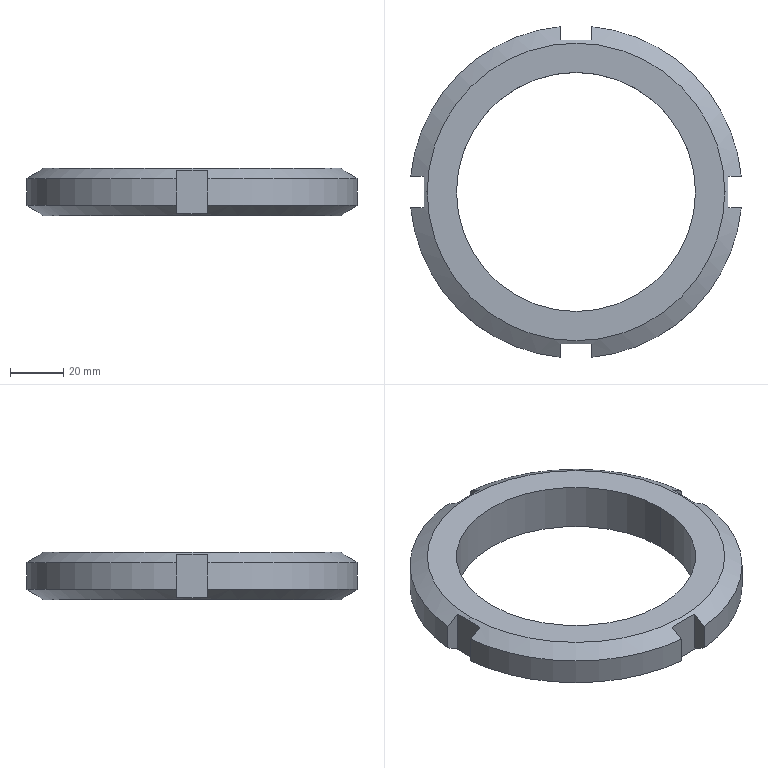Part | SolidWorks | features Extrusion 1, ICE 1, RevCut 1 | 1 solid | 24 faces | box 124.423 x 124.423 x 18 mm | volume 93238 mm3 | plane 14 | cylinder 6 | cone 4 | commonest cylinder face diameters 125 x4 90 x2
STEP:
#1=CARTESIAN_POINT('',(-56.,0.,18.));
#2=VERTEX_POINT('',#1);
#3=CARTESIAN_POINT('',(56.,0.,18.));
#4=VERTEX_POINT('',#3);
#5=CARTESIAN_POINT('',(0.,0.,18.));
#6=DIRECTION('',(0.,0.,-1.));
#7=DIRECTION('',(-1.,0.,0.));
#8=AXIS2_PLACEMENT_3D('',#5,#6,#7);
#9=CIRCLE('',#8,56.);
#10=EDGE_CURVE('',#2,#4,#9,.T.);
#11=ORIENTED_EDGE('',*,*,#10,.T.);
#12=CARTESIAN_POINT('',(57.211,0.,17.255));
#13=VERTEX_POINT('',#12);
#14=CARTESIAN_POINT('',(62.5,0.,14.));
#15=DIRECTION('',(0.8517,0.,-0.5241));
#16=VECTOR('',#15,1000.);
#17=LINE('',#14,#16);
#18=EDGE_CURVE('',#4,#13,#17,.T.);
#19=ORIENTED_EDGE('',*,*,#18,.T.);
#20=CARTESIAN_POINT('',(57.211,6.,17.061));
#21=VERTEX_POINT('',#20);
#22=CARTESIAN_POINT('',(57.211,6.,17.061));
#23=CARTESIAN_POINT('',(57.211,4.005,17.19));
#24=CARTESIAN_POINT('',(57.211,2.005,17.255));
#25=CARTESIAN_POINT('',(57.211,0.,17.255));
#26=B_SPLINE_CURVE_WITH_KNOTS('',3,(#22,#23,#24,#25),.UNSPECIFIED.,.F.,.F.,(4,4),(0.0144,0.02039),.UNSPECIFIED.);
#27=EDGE_CURVE('',#21,#13,#26,.T.);
#28=ORIENTED_EDGE('',*,*,#27,.F.);
#29=CARTESIAN_POINT('',(62.211,6.,14.));
#30=VERTEX_POINT('',#29);
#31=CARTESIAN_POINT('',(62.211,6.,14.));
#32=CARTESIAN_POINT('',(61.305,6.,14.555));
#33=CARTESIAN_POINT('',(60.399,6.,15.11));
#34=CARTESIAN_POINT('',(59.493,6.,15.665));
#35=CARTESIAN_POINT('',(58.733,6.,16.13));
#36=CARTESIAN_POINT('',(57.972,6.,16.596));
#37=CARTESIAN_POINT('',(57.211,6.,17.061));
#38=B_SPLINE_CURVE_WITH_KNOTS('',3,(#31,#32,#33,#34,#35,#36,#37),.UNSPECIFIED.,.F.,.F.,(4,3,4),(0.008854,0.01204,0.01472),.UNSPECIFIED.);
#39=EDGE_CURVE('',#30,#21,#38,.T.);
#40=ORIENTED_EDGE('',*,*,#39,.F.);
#41=CARTESIAN_POINT('',(6.,62.211,14.));
#42=VERTEX_POINT('',#41);
#43=CARTESIAN_POINT('',(0.,0.,14.));
#44=DIRECTION('',(0.,0.,-1.));
#45=DIRECTION('',(-1.,0.,0.));
#46=AXIS2_PLACEMENT_3D('',#43,#44,#45);
#47=CIRCLE('',#46,62.5);
#48=EDGE_CURVE('',#42,#30,#47,.T.);
#49=ORIENTED_EDGE('',*,*,#48,.F.);
#50=CARTESIAN_POINT('',(6.,57.211,17.061));
#51=VERTEX_POINT('',#50);
#52=CARTESIAN_POINT('',(6.,57.211,17.061));
#53=CARTESIAN_POINT('',(6.,57.972,16.596));
#54=CARTESIAN_POINT('',(6.,58.733,16.13));
#55=CARTESIAN_POINT('',(6.,59.493,15.665));
#56=CARTESIAN_POINT('',(6.,60.399,15.11));
#57=CARTESIAN_POINT('',(6.,61.305,14.555));
#58=CARTESIAN_POINT('',(6.,62.211,14.));
#59=B_SPLINE_CURVE_WITH_KNOTS('',3,(#52,#53,#54,#55,#56,#57,#58),.UNSPECIFIED.,.F.,.F.,(4,3,4),(0.009366,0.01204,0.01523),.UNSPECIFIED.);
#60=EDGE_CURVE('',#51,#42,#59,.T.);
#61=ORIENTED_EDGE('',*,*,#60,.F.);
#62=CARTESIAN_POINT('',(-6.,57.211,17.061));
#63=VERTEX_POINT('',#62);
#64=CARTESIAN_POINT('',(-6.,57.211,17.061));
#65=CARTESIAN_POINT('',(-4.998,57.211,17.126));
#66=CARTESIAN_POINT('',(-3.993,57.211,17.174));
#67=CARTESIAN_POINT('',(-1.987,57.211,17.239));
#68=CARTESIAN_POINT('',(-0.9858,57.211,17.255));
#69=CARTESIAN_POINT('',(2.015,57.211,17.254));
#70=CARTESIAN_POINT('',(4.01,57.211,17.189));
#71=CARTESIAN_POINT('',(6.,57.211,17.061));
#72=B_SPLINE_CURVE_WITH_KNOTS('',3,(#64,#65,#66,#67,#68,#69,#70,#71),.UNSPECIFIED.,.F.,.F.,(4,2,2,4),(0.02345,0.02644,0.02944,0.03543),.UNSPECIFIED.);
#73=EDGE_CURVE('',#63,#51,#72,.T.);
#74=ORIENTED_EDGE('',*,*,#73,.F.);
#75=CARTESIAN_POINT('',(-6.,62.211,14.));
#76=VERTEX_POINT('',#75);
#77=CARTESIAN_POINT('',(-6.,62.211,14.));
#78=CARTESIAN_POINT('',(-6.,61.305,14.555));
#79=CARTESIAN_POINT('',(-6.,60.399,15.11));
#80=CARTESIAN_POINT('',(-6.,59.493,15.665));
#81=CARTESIAN_POINT('',(-6.,58.733,16.13));
#82=CARTESIAN_POINT('',(-6.,57.972,16.596));
#83=CARTESIAN_POINT('',(-6.,57.211,17.061));
#84=B_SPLINE_CURVE_WITH_KNOTS('',3,(#77,#78,#79,#80,#81,#82,#83),.UNSPECIFIED.,.F.,.F.,(4,3,4),(0.008854,0.01204,0.01472),.UNSPECIFIED.);
#85=EDGE_CURVE('',#76,#63,#84,.T.);
#86=ORIENTED_EDGE('',*,*,#85,.F.);
#87=CARTESIAN_POINT('',(-62.211,6.,14.));
#88=VERTEX_POINT('',#87);
#89=CARTESIAN_POINT('',(0.,0.,14.));
#90=DIRECTION('',(0.,0.,-1.));
#91=DIRECTION('',(-1.,0.,0.));
#92=AXIS2_PLACEMENT_3D('',#89,#90,#91);
#93=CIRCLE('',#92,62.5);
#94=EDGE_CURVE('',#88,#76,#93,.T.);
#95=ORIENTED_EDGE('',*,*,#94,.F.);
#96=CARTESIAN_POINT('',(-57.211,6.,17.061));
#97=VERTEX_POINT('',#96);
#98=CARTESIAN_POINT('',(-57.211,6.,17.061));
#99=CARTESIAN_POINT('',(-58.578,6.,16.225));
#100=CARTESIAN_POINT('',(-59.945,6.,15.388));
#101=CARTESIAN_POINT('',(-61.311,6.,14.551));
#102=CARTESIAN_POINT('',(-61.611,6.,14.367));
#103=CARTESIAN_POINT('',(-61.911,6.,14.184));
#104=CARTESIAN_POINT('',(-62.211,6.,14.));
#105=B_SPLINE_CURVE_WITH_KNOTS('',3,(#98,#99,#100,#101,#102,#103,#104),.UNSPECIFIED.,.F.,.F.,(4,3,4),(0.007234,0.01204,0.0131),.UNSPECIFIED.);
#106=EDGE_CURVE('',#97,#88,#105,.T.);
#107=ORIENTED_EDGE('',*,*,#106,.F.);
#108=CARTESIAN_POINT('',(-57.211,0.,17.255));
#109=VERTEX_POINT('',#108);
#110=CARTESIAN_POINT('',(-57.211,0.,17.255));
#111=CARTESIAN_POINT('',(-57.211,2.005,17.255));
#112=CARTESIAN_POINT('',(-57.211,4.005,17.19));
#113=CARTESIAN_POINT('',(-57.211,6.,17.061));
#114=B_SPLINE_CURVE_WITH_KNOTS('',3,(#110,#111,#112,#113),.UNSPECIFIED.,.F.,.F.,(4,4),(0.02943,0.03543),.UNSPECIFIED.);
#115=EDGE_CURVE('',#109,#97,#114,.T.);
#116=ORIENTED_EDGE('',*,*,#115,.F.);
#117=CARTESIAN_POINT('',(-62.5,0.,14.));
#118=DIRECTION('',(-0.8517,0.,-0.5241));
#119=VECTOR('',#118,1000.);
#120=LINE('',#117,#119);
#121=EDGE_CURVE('',#2,#109,#120,.T.);
#122=ORIENTED_EDGE('',*,*,#121,.F.);
#123=EDGE_LOOP('',(#11,#19,#28,#40,#49,#61,#74,#86,#95,#107,#116,#122));
#124=FACE_OUTER_BOUND('',#123,.T.);
#125=CARTESIAN_POINT('',(0.,0.,14.));
#126=DIRECTION('',(0.,0.,-1.));
#127=DIRECTION('',(-1.,0.,0.));
#128=AXIS2_PLACEMENT_3D('',#125,#126,#127);
#129=CONICAL_SURFACE('',#128,62.5,1.019);
#130=ADVANCED_FACE('',(#124),#129,.T.);
#131=CARTESIAN_POINT('',(-56.,0.,0.));
#132=VERTEX_POINT('',#131);
#133=CARTESIAN_POINT('',(56.,0.,0.));
#134=VERTEX_POINT('',#133);
#135=CARTESIAN_POINT('',(0.,0.,0.));
#136=DIRECTION('',(0.,0.,-1.));
#137=DIRECTION('',(-1.,0.,0.));
#138=AXIS2_PLACEMENT_3D('',#135,#136,#137);
#139=CIRCLE('',#138,56.);
#140=EDGE_CURVE('',#132,#134,#139,.T.);
#141=ORIENTED_EDGE('',*,*,#140,.F.);
#142=CARTESIAN_POINT('',(-57.211,0.,0.7454));
#143=VERTEX_POINT('',#142);
#144=CARTESIAN_POINT('',(-56.,0.,0.));
#145=DIRECTION('',(-0.8517,0.,0.5241));
#146=VECTOR('',#145,1000.);
#147=LINE('',#144,#146);
#148=EDGE_CURVE('',#132,#143,#147,.T.);
#149=ORIENTED_EDGE('',*,*,#148,.T.);
#150=CARTESIAN_POINT('',(-57.211,6.,0.9385));
#151=VERTEX_POINT('',#150);
#152=CARTESIAN_POINT('',(-57.211,6.,0.9385));
#153=CARTESIAN_POINT('',(-57.211,4.005,0.8105));
#154=CARTESIAN_POINT('',(-57.211,2.005,0.7454));
#155=CARTESIAN_POINT('',(-57.211,0.,0.7454));
#156=B_SPLINE_CURVE_WITH_KNOTS('',3,(#152,#153,#154,#155),.UNSPECIFIED.,.F.,.F.,(4,4),(0.0144,0.02039),.UNSPECIFIED.);
#157=EDGE_CURVE('',#151,#143,#156,.T.);
#158=ORIENTED_EDGE('',*,*,#157,.F.);
#159=CARTESIAN_POINT('',(-62.211,6.,4.));
#160=VERTEX_POINT('',#159);
#161=CARTESIAN_POINT('',(-62.211,6.,4.));
#162=CARTESIAN_POINT('',(-61.911,6.,3.816));
#163=CARTESIAN_POINT('',(-61.611,6.,3.633));
#164=CARTESIAN_POINT('',(-61.311,6.,3.449));
#165=CARTESIAN_POINT('',(-59.945,6.,2.612));
#166=CARTESIAN_POINT('',(-58.578,6.,1.775));
#167=CARTESIAN_POINT('',(-57.211,6.,0.9385));
#168=B_SPLINE_CURVE_WITH_KNOTS('',3,(#161,#162,#163,#164,#165,#166,#167),.UNSPECIFIED.,.F.,.F.,(4,3,4),(0.01099,0.01204,0.01685),.UNSPECIFIED.);
#169=EDGE_CURVE('',#160,#151,#168,.T.);
#170=ORIENTED_EDGE('',*,*,#169,.F.);
#171=CARTESIAN_POINT('',(-6.,62.211,4.));
#172=VERTEX_POINT('',#171);
#173=CARTESIAN_POINT('',(0.,0.,4.));
#174=DIRECTION('',(0.,0.,-1.));
#175=DIRECTION('',(-1.,0.,0.));
#176=AXIS2_PLACEMENT_3D('',#173,#174,#175);
#177=CIRCLE('',#176,62.5);
#178=EDGE_CURVE('',#160,#172,#177,.T.);
#179=ORIENTED_EDGE('',*,*,#178,.T.);
#180=CARTESIAN_POINT('',(-6.,57.211,0.9385));
#181=VERTEX_POINT('',#180);
#182=CARTESIAN_POINT('',(-6.,57.211,0.9385));
#183=CARTESIAN_POINT('',(-6.,57.372,1.037));
#184=CARTESIAN_POINT('',(-6.,57.533,1.135));
#185=CARTESIAN_POINT('',(-6.,57.693,1.234));
#186=CARTESIAN_POINT('',(-6.,59.2,2.155));
#187=CARTESIAN_POINT('',(-6.,60.705,3.078));
#188=CARTESIAN_POINT('',(-6.,62.211,4.));
#189=B_SPLINE_CURVE_WITH_KNOTS('',3,(#182,#183,#184,#185,#186,#187,#188),.UNSPECIFIED.,.F.,.F.,(4,3,4),(0.01148,0.01204,0.01734),.UNSPECIFIED.);
#190=EDGE_CURVE('',#181,#172,#189,.T.);
#191=ORIENTED_EDGE('',*,*,#190,.F.);
#192=CARTESIAN_POINT('',(6.,57.211,0.9385));
#193=VERTEX_POINT('',#192);
#194=CARTESIAN_POINT('',(6.,57.211,0.9385));
#195=CARTESIAN_POINT('',(4.01,57.211,0.8108));
#196=CARTESIAN_POINT('',(2.015,57.211,0.7457));
#197=CARTESIAN_POINT('',(-0.9858,57.211,0.7453));
#198=CARTESIAN_POINT('',(-1.987,57.211,0.7613));
#199=CARTESIAN_POINT('',(-3.993,57.211,0.8257));
#200=CARTESIAN_POINT('',(-4.998,57.211,0.8742));
#201=CARTESIAN_POINT('',(-6.,57.211,0.9385));
#202=B_SPLINE_CURVE_WITH_KNOTS('',3,(#194,#195,#196,#197,#198,#199,#200,#201),.UNSPECIFIED.,.F.,.F.,(4,2,2,4),(0.0144,0.02038,0.02337,0.02636),.UNSPECIFIED.);
#203=EDGE_CURVE('',#193,#181,#202,.T.);
#204=ORIENTED_EDGE('',*,*,#203,.F.);
#205=CARTESIAN_POINT('',(6.,62.211,4.));
#206=VERTEX_POINT('',#205);
#207=CARTESIAN_POINT('',(6.,62.211,4.));
#208=CARTESIAN_POINT('',(6.,60.705,3.078));
#209=CARTESIAN_POINT('',(6.,59.2,2.155));
#210=CARTESIAN_POINT('',(6.,57.693,1.234));
#211=CARTESIAN_POINT('',(6.,57.533,1.135));
#212=CARTESIAN_POINT('',(6.,57.372,1.037));
#213=CARTESIAN_POINT('',(6.,57.211,0.9385));
#214=B_SPLINE_CURVE_WITH_KNOTS('',3,(#207,#208,#209,#210,#211,#212,#213),.UNSPECIFIED.,.F.,.F.,(4,3,4),(0.006744,0.01204,0.01261),.UNSPECIFIED.);
#215=EDGE_CURVE('',#206,#193,#214,.T.);
#216=ORIENTED_EDGE('',*,*,#215,.F.);
#217=CARTESIAN_POINT('',(62.211,6.,4.));
#218=VERTEX_POINT('',#217);
#219=CARTESIAN_POINT('',(0.,0.,4.));
#220=DIRECTION('',(0.,0.,-1.));
#221=DIRECTION('',(-1.,0.,0.));
#222=AXIS2_PLACEMENT_3D('',#219,#220,#221);
#223=CIRCLE('',#222,62.5);
#224=EDGE_CURVE('',#206,#218,#223,.T.);
#225=ORIENTED_EDGE('',*,*,#224,.T.);
#226=CARTESIAN_POINT('',(57.211,6.,0.9385));
#227=VERTEX_POINT('',#226);
#228=CARTESIAN_POINT('',(57.211,6.,0.9385));
#229=CARTESIAN_POINT('',(57.372,6.,1.037));
#230=CARTESIAN_POINT('',(57.533,6.,1.135));
#231=CARTESIAN_POINT('',(57.693,6.,1.234));
#232=CARTESIAN_POINT('',(59.2,6.,2.155));
#233=CARTESIAN_POINT('',(60.705,6.,3.078));
#234=CARTESIAN_POINT('',(62.211,6.,4.));
#235=B_SPLINE_CURVE_WITH_KNOTS('',3,(#228,#229,#230,#231,#232,#233,#234),.UNSPECIFIED.,.F.,.F.,(4,3,4),(0.01148,0.01204,0.01734),.UNSPECIFIED.);
#236=EDGE_CURVE('',#227,#218,#235,.T.);
#237=ORIENTED_EDGE('',*,*,#236,.F.);
#238=CARTESIAN_POINT('',(57.211,0.,0.7454));
#239=VERTEX_POINT('',#238);
#240=CARTESIAN_POINT('',(57.211,0.,0.7454));
#241=CARTESIAN_POINT('',(57.211,2.005,0.7454));
#242=CARTESIAN_POINT('',(57.211,4.005,0.8105));
#243=CARTESIAN_POINT('',(57.211,6.,0.9385));
#244=B_SPLINE_CURVE_WITH_KNOTS('',3,(#240,#241,#242,#243),.UNSPECIFIED.,.F.,.F.,(4,4),(0.02943,0.03543),.UNSPECIFIED.);
#245=EDGE_CURVE('',#239,#227,#244,.T.);
#246=ORIENTED_EDGE('',*,*,#245,.F.);
#247=CARTESIAN_POINT('',(56.,0.,0.));
#248=DIRECTION('',(0.8517,0.,0.5241));
#249=VECTOR('',#248,1000.);
#250=LINE('',#247,#249);
#251=EDGE_CURVE('',#134,#239,#250,.T.);
#252=ORIENTED_EDGE('',*,*,#251,.F.);
#253=EDGE_LOOP('',(#141,#149,#158,#170,#179,#191,#204,#216,#225,#237,#246,#252));
#254=FACE_OUTER_BOUND('',#253,.T.);
#255=CARTESIAN_POINT('',(0.,0.,0.));
#256=DIRECTION('',(0.,0.,1.));
#257=DIRECTION('',(1.,0.,0.));
#258=AXIS2_PLACEMENT_3D('',#255,#256,#257);
#259=CONICAL_SURFACE('',#258,56.,1.019);
#260=ADVANCED_FACE('',(#254),#259,.T.);
#261=CARTESIAN_POINT('',(-45.,0.,18.));
#262=VERTEX_POINT('',#261);
#263=CARTESIAN_POINT('',(45.,0.,18.));
#264=VERTEX_POINT('',#263);
#265=CARTESIAN_POINT('',(0.,0.,18.));
#266=DIRECTION('',(0.,0.,1.));
#267=DIRECTION('',(1.,0.,0.));
#268=AXIS2_PLACEMENT_3D('',#265,#266,#267);
#269=CIRCLE('',#268,45.);
#270=EDGE_CURVE('',#262,#264,#269,.T.);
#271=ORIENTED_EDGE('',*,*,#270,.T.);
#272=CARTESIAN_POINT('',(45.,0.,0.));
#273=VERTEX_POINT('',#272);
#274=CARTESIAN_POINT('',(45.,0.,18.));
#275=DIRECTION('',(0.,0.,-1.));
#276=VECTOR('',#275,1000.);
#277=LINE('',#274,#276);
#278=EDGE_CURVE('',#264,#273,#277,.T.);
#279=ORIENTED_EDGE('',*,*,#278,.T.);
#280=CARTESIAN_POINT('',(-45.,0.,0.));
#281=VERTEX_POINT('',#280);
#282=CARTESIAN_POINT('',(0.,0.,0.));
#283=DIRECTION('',(0.,0.,1.));
#284=DIRECTION('',(1.,0.,0.));
#285=AXIS2_PLACEMENT_3D('',#282,#283,#284);
#286=CIRCLE('',#285,45.);
#287=EDGE_CURVE('',#281,#273,#286,.T.);
#288=ORIENTED_EDGE('',*,*,#287,.F.);
#289=CARTESIAN_POINT('',(-45.,0.,18.));
#290=DIRECTION('',(0.,0.,-1.));
#291=VECTOR('',#290,1000.);
#292=LINE('',#289,#291);
#293=EDGE_CURVE('',#262,#281,#292,.T.);
#294=ORIENTED_EDGE('',*,*,#293,.F.);
#295=EDGE_LOOP('',(#271,#279,#288,#294));
#296=FACE_OUTER_BOUND('',#295,.T.);
#297=CARTESIAN_POINT('',(0.,0.,18.));
#298=DIRECTION('',(0.,0.,-1.));
#299=DIRECTION('',(-1.,0.,0.));
#300=AXIS2_PLACEMENT_3D('',#297,#298,#299);
#301=CYLINDRICAL_SURFACE('',#300,45.);
#302=ADVANCED_FACE('',(#296),#301,.F.);
#303=CARTESIAN_POINT('',(-6.,-62.211,14.));
#304=VERTEX_POINT('',#303);
#305=CARTESIAN_POINT('',(-62.211,-6.,14.));
#306=VERTEX_POINT('',#305);
#307=CARTESIAN_POINT('',(0.,0.,14.));
#308=DIRECTION('',(0.,0.,-1.));
#309=DIRECTION('',(-1.,0.,0.));
#310=AXIS2_PLACEMENT_3D('',#307,#308,#309);
#311=CIRCLE('',#310,62.5);
#312=EDGE_CURVE('',#304,#306,#311,.T.);
#313=ORIENTED_EDGE('',*,*,#312,.T.);
#314=CARTESIAN_POINT('',(-62.211,-6.,4.));
#315=VERTEX_POINT('',#314);
#316=CARTESIAN_POINT('',(-62.211,-6.,18.));
#317=DIRECTION('',(0.,0.,-1.));
#318=VECTOR('',#317,1000.);
#319=LINE('',#316,#318);
#320=EDGE_CURVE('',#306,#315,#319,.T.);
#321=ORIENTED_EDGE('',*,*,#320,.T.);
#322=CARTESIAN_POINT('',(-6.,-62.211,4.));
#323=VERTEX_POINT('',#322);
#324=CARTESIAN_POINT('',(0.,0.,4.));
#325=DIRECTION('',(0.,0.,-1.));
#326=DIRECTION('',(-1.,0.,0.));
#327=AXIS2_PLACEMENT_3D('',#324,#325,#326);
#328=CIRCLE('',#327,62.5);
#329=EDGE_CURVE('',#323,#315,#328,.T.);
#330=ORIENTED_EDGE('',*,*,#329,.F.);
#331=CARTESIAN_POINT('',(-6.,-62.211,18.));
#332=DIRECTION('',(0.,0.,-1.));
#333=VECTOR('',#332,1000.);
#334=LINE('',#331,#333);
#335=EDGE_CURVE('',#304,#323,#334,.T.);
#336=ORIENTED_EDGE('',*,*,#335,.F.);
#337=EDGE_LOOP('',(#313,#321,#330,#336));
#338=FACE_OUTER_BOUND('',#337,.T.);
#339=CARTESIAN_POINT('',(0.,0.,18.));
#340=DIRECTION('',(0.,0.,-1.));
#341=DIRECTION('',(-1.,0.,0.));
#342=AXIS2_PLACEMENT_3D('',#339,#340,#341);
#343=CYLINDRICAL_SURFACE('',#342,62.5);
#344=ADVANCED_FACE('',(#338),#343,.T.);
#345=CARTESIAN_POINT('',(62.211,-6.,14.));
#346=VERTEX_POINT('',#345);
#347=CARTESIAN_POINT('',(6.,-62.211,14.));
#348=VERTEX_POINT('',#347);
#349=CARTESIAN_POINT('',(0.,0.,14.));
#350=DIRECTION('',(0.,0.,-1.));
#351=DIRECTION('',(-1.,0.,0.));
#352=AXIS2_PLACEMENT_3D('',#349,#350,#351);
#353=CIRCLE('',#352,62.5);
#354=EDGE_CURVE('',#346,#348,#353,.T.);
#355=ORIENTED_EDGE('',*,*,#354,.T.);
#356=CARTESIAN_POINT('',(6.,-62.211,4.));
#357=VERTEX_POINT('',#356);
#358=CARTESIAN_POINT('',(6.,-62.211,18.));
#359=DIRECTION('',(0.,0.,-1.));
#360=VECTOR('',#359,1000.);
#361=LINE('',#358,#360);
#362=EDGE_CURVE('',#348,#357,#361,.T.);
#363=ORIENTED_EDGE('',*,*,#362,.T.);
#364=CARTESIAN_POINT('',(62.211,-6.,4.));
#365=VERTEX_POINT('',#364);
#366=CARTESIAN_POINT('',(0.,0.,4.));
#367=DIRECTION('',(0.,0.,-1.));
#368=DIRECTION('',(-1.,0.,0.));
#369=AXIS2_PLACEMENT_3D('',#366,#367,#368);
#370=CIRCLE('',#369,62.5);
#371=EDGE_CURVE('',#365,#357,#370,.T.);
#372=ORIENTED_EDGE('',*,*,#371,.F.);
#373=CARTESIAN_POINT('',(62.211,-6.,18.));
#374=DIRECTION('',(0.,0.,-1.));
#375=VECTOR('',#374,1000.);
#376=LINE('',#373,#375);
#377=EDGE_CURVE('',#346,#365,#376,.T.);
#378=ORIENTED_EDGE('',*,*,#377,.F.);
#379=EDGE_LOOP('',(#355,#363,#372,#378));
#380=FACE_OUTER_BOUND('',#379,.T.);
#381=CARTESIAN_POINT('',(0.,0.,18.));
#382=DIRECTION('',(0.,0.,-1.));
#383=DIRECTION('',(-1.,0.,0.));
#384=AXIS2_PLACEMENT_3D('',#381,#382,#383);
#385=CYLINDRICAL_SURFACE('',#384,62.5);
#386=ADVANCED_FACE('',(#380),#385,.T.);
#387=ORIENTED_EDGE('',*,*,#48,.T.);
#388=CARTESIAN_POINT('',(62.211,6.,18.));
#389=DIRECTION('',(0.,0.,-1.));
#390=VECTOR('',#389,1000.);
#391=LINE('',#388,#390);
#392=EDGE_CURVE('',#30,#218,#391,.T.);
#393=ORIENTED_EDGE('',*,*,#392,.T.);
#394=ORIENTED_EDGE('',*,*,#224,.F.);
#395=CARTESIAN_POINT('',(6.,62.211,18.));
#396=DIRECTION('',(0.,0.,-1.));
#397=VECTOR('',#396,1000.);
#398=LINE('',#395,#397);
#399=EDGE_CURVE('',#42,#206,#398,.T.);
#400=ORIENTED_EDGE('',*,*,#399,.F.);
#401=EDGE_LOOP('',(#387,#393,#394,#400));
#402=FACE_OUTER_BOUND('',#401,.T.);
#403=CARTESIAN_POINT('',(0.,0.,18.));
#404=DIRECTION('',(0.,0.,-1.));
#405=DIRECTION('',(-1.,0.,0.));
#406=AXIS2_PLACEMENT_3D('',#403,#404,#405);
#407=CYLINDRICAL_SURFACE('',#406,62.5);
#408=ADVANCED_FACE('',(#402),#407,.T.);
#409=ORIENTED_EDGE('',*,*,#178,.F.);
#410=CARTESIAN_POINT('',(-62.211,6.,18.));
#411=DIRECTION('',(0.,0.,-1.));
#412=VECTOR('',#411,1000.);
#413=LINE('',#410,#412);
#414=EDGE_CURVE('',#88,#160,#413,.T.);
#415=ORIENTED_EDGE('',*,*,#414,.F.);
#416=ORIENTED_EDGE('',*,*,#94,.T.);
#417=CARTESIAN_POINT('',(-6.,62.211,18.));
#418=DIRECTION('',(0.,0.,-1.));
#419=VECTOR('',#418,1000.);
#420=LINE('',#417,#419);
#421=EDGE_CURVE('',#76,#172,#420,.T.);
#422=ORIENTED_EDGE('',*,*,#421,.T.);
#423=EDGE_LOOP('',(#409,#415,#416,#422));
#424=FACE_OUTER_BOUND('',#423,.T.);
#425=CARTESIAN_POINT('',(0.,0.,18.));
#426=DIRECTION('',(0.,0.,-1.));
#427=DIRECTION('',(-1.,0.,0.));
#428=AXIS2_PLACEMENT_3D('',#425,#426,#427);
#429=CYLINDRICAL_SURFACE('',#428,62.5);
#430=ADVANCED_FACE('',(#424),#429,.T.);
#431=ORIENTED_EDGE('',*,*,#270,.F.);
#432=CARTESIAN_POINT('',(0.,0.,18.));
#433=DIRECTION('',(0.,0.,1.));
#434=DIRECTION('',(1.,0.,0.));
#435=AXIS2_PLACEMENT_3D('',#432,#433,#434);
#436=CIRCLE('',#435,45.);
#437=EDGE_CURVE('',#264,#262,#436,.T.);
#438=ORIENTED_EDGE('',*,*,#437,.F.);
#439=EDGE_LOOP('',(#431,#438));
#440=FACE_BOUND('',#439,.T.);
#441=ORIENTED_EDGE('',*,*,#10,.F.);
#442=CARTESIAN_POINT('',(0.,0.,18.));
#443=DIRECTION('',(0.,0.,-1.));
#444=DIRECTION('',(-1.,0.,0.));
#445=AXIS2_PLACEMENT_3D('',#442,#443,#444);
#446=CIRCLE('',#445,56.);
#447=EDGE_CURVE('',#4,#2,#446,.T.);
#448=ORIENTED_EDGE('',*,*,#447,.F.);
#449=EDGE_LOOP('',(#441,#448));
#450=FACE_OUTER_BOUND('',#449,.T.);
#451=CARTESIAN_POINT('',(0.,0.,18.));
#452=DIRECTION('',(0.,0.,1.));
#453=DIRECTION('',(1.,0.,0.));
#454=AXIS2_PLACEMENT_3D('',#451,#452,#453);
#455=PLANE('',#454);
#456=ADVANCED_FACE('',(#440,#450),#455,.T.);
#457=ORIENTED_EDGE('',*,*,#287,.T.);
#458=CARTESIAN_POINT('',(0.,0.,0.));
#459=DIRECTION('',(0.,0.,1.));
#460=DIRECTION('',(1.,0.,0.));
#461=AXIS2_PLACEMENT_3D('',#458,#459,#460);
#462=CIRCLE('',#461,45.);
#463=EDGE_CURVE('',#273,#281,#462,.T.);
#464=ORIENTED_EDGE('',*,*,#463,.T.);
#465=EDGE_LOOP('',(#457,#464));
#466=FACE_BOUND('',#465,.T.);
#467=CARTESIAN_POINT('',(0.,0.,0.));
#468=DIRECTION('',(0.,0.,-1.));
#469=DIRECTION('',(-1.,0.,0.));
#470=AXIS2_PLACEMENT_3D('',#467,#468,#469);
#471=CIRCLE('',#470,56.);
#472=EDGE_CURVE('',#134,#132,#471,.T.);
#473=ORIENTED_EDGE('',*,*,#472,.T.);
#474=ORIENTED_EDGE('',*,*,#140,.T.);
#475=EDGE_LOOP('',(#473,#474));
#476=FACE_OUTER_BOUND('',#475,.T.);
#477=CARTESIAN_POINT('',(0.,0.,0.));
#478=DIRECTION('',(0.,0.,1.));
#479=DIRECTION('',(1.,0.,0.));
#480=AXIS2_PLACEMENT_3D('',#477,#478,#479);
#481=PLANE('',#480);
#482=ADVANCED_FACE('',(#466,#476),#481,.F.);
#483=ORIENTED_EDGE('',*,*,#278,.F.);
#484=ORIENTED_EDGE('',*,*,#437,.T.);
#485=ORIENTED_EDGE('',*,*,#293,.T.);
#486=ORIENTED_EDGE('',*,*,#463,.F.);
#487=EDGE_LOOP('',(#483,#484,#485,#486));
#488=FACE_OUTER_BOUND('',#487,.T.);
#489=CARTESIAN_POINT('',(0.,0.,18.));
#490=DIRECTION('',(0.,0.,-1.));
#491=DIRECTION('',(-1.,0.,0.));
#492=AXIS2_PLACEMENT_3D('',#489,#490,#491);
#493=CYLINDRICAL_SURFACE('',#492,45.);
#494=ADVANCED_FACE('',(#488),#493,.F.);
#495=ORIENTED_EDGE('',*,*,#148,.F.);
#496=ORIENTED_EDGE('',*,*,#472,.F.);
#497=ORIENTED_EDGE('',*,*,#251,.T.);
#498=CARTESIAN_POINT('',(57.211,-6.,0.9385));
#499=VERTEX_POINT('',#498);
#500=CARTESIAN_POINT('',(57.211,-6.,0.9385));
#501=CARTESIAN_POINT('',(57.211,-5.001,0.8744));
#502=CARTESIAN_POINT('',(57.211,-3.998,0.8259));
#503=CARTESIAN_POINT('',(57.211,-1.997,0.7615));
#504=CARTESIAN_POINT('',(57.211,-0.9978,0.7454));
#505=CARTESIAN_POINT('',(57.211,0.,0.7454));
#506=B_SPLINE_CURVE_WITH_KNOTS('',3,(#500,#501,#502,#503,#504,#505),.UNSPECIFIED.,.F.,.F.,(4,2,4),(0.02345,0.02644,0.02943),.UNSPECIFIED.);
#507=EDGE_CURVE('',#499,#239,#506,.T.);
#508=ORIENTED_EDGE('',*,*,#507,.F.);
#509=CARTESIAN_POINT('',(62.211,-6.,4.));
#510=CARTESIAN_POINT('',(60.705,-6.,3.078));
#511=CARTESIAN_POINT('',(59.2,-6.,2.155));
#512=CARTESIAN_POINT('',(57.693,-6.,1.234));
#513=CARTESIAN_POINT('',(57.533,-6.,1.135));
#514=CARTESIAN_POINT('',(57.372,-6.,1.037));
#515=CARTESIAN_POINT('',(57.211,-6.,0.9385));
#516=B_SPLINE_CURVE_WITH_KNOTS('',3,(#509,#510,#511,#512,#513,#514,#515),.UNSPECIFIED.,.F.,.F.,(4,3,4),(0.006744,0.01204,0.01261),.UNSPECIFIED.);
#517=EDGE_CURVE('',#365,#499,#516,.T.);
#518=ORIENTED_EDGE('',*,*,#517,.F.);
#519=ORIENTED_EDGE('',*,*,#371,.T.);
#520=CARTESIAN_POINT('',(6.,-57.211,0.9385));
#521=VERTEX_POINT('',#520);
#522=CARTESIAN_POINT('',(6.,-57.211,0.9385));
#523=CARTESIAN_POINT('',(6.,-58.578,1.775));
#524=CARTESIAN_POINT('',(6.,-59.945,2.612));
#525=CARTESIAN_POINT('',(6.,-61.311,3.449));
#526=CARTESIAN_POINT('',(6.,-61.611,3.633));
#527=CARTESIAN_POINT('',(6.,-61.911,3.816));
#528=CARTESIAN_POINT('',(6.,-62.211,4.));
#529=B_SPLINE_CURVE_WITH_KNOTS('',3,(#522,#523,#524,#525,#526,#527,#528),.UNSPECIFIED.,.F.,.F.,(4,3,4),(0.007234,0.01204,0.0131),.UNSPECIFIED.);
#530=EDGE_CURVE('',#521,#357,#529,.T.);
#531=ORIENTED_EDGE('',*,*,#530,.F.);
#532=CARTESIAN_POINT('',(-6.,-57.211,0.9385));
#533=VERTEX_POINT('',#532);
#534=CARTESIAN_POINT('',(-6.,-57.211,0.9385));
#535=CARTESIAN_POINT('',(-4.998,-57.211,0.8742));
#536=CARTESIAN_POINT('',(-3.993,-57.211,0.8257));
#537=CARTESIAN_POINT('',(-1.987,-57.211,0.7613));
#538=CARTESIAN_POINT('',(-0.9858,-57.211,0.7453));
#539=CARTESIAN_POINT('',(2.015,-57.211,0.7457));
#540=CARTESIAN_POINT('',(4.01,-57.211,0.8108));
#541=CARTESIAN_POINT('',(6.,-57.211,0.9385));
#542=B_SPLINE_CURVE_WITH_KNOTS('',3,(#534,#535,#536,#537,#538,#539,#540,#541),.UNSPECIFIED.,.F.,.F.,(4,2,2,4),(0.02345,0.02644,0.02944,0.03543),.UNSPECIFIED.);
#543=EDGE_CURVE('',#533,#521,#542,.T.);
#544=ORIENTED_EDGE('',*,*,#543,.F.);
#545=CARTESIAN_POINT('',(-6.,-62.211,4.));
#546=CARTESIAN_POINT('',(-6.,-61.911,3.816));
#547=CARTESIAN_POINT('',(-6.,-61.611,3.633));
#548=CARTESIAN_POINT('',(-6.,-61.311,3.449));
#549=CARTESIAN_POINT('',(-6.,-59.945,2.612));
#550=CARTESIAN_POINT('',(-6.,-58.578,1.775));
#551=CARTESIAN_POINT('',(-6.,-57.211,0.9385));
#552=B_SPLINE_CURVE_WITH_KNOTS('',3,(#545,#546,#547,#548,#549,#550,#551),.UNSPECIFIED.,.F.,.F.,(4,3,4),(0.01099,0.01204,0.01685),.UNSPECIFIED.);
#553=EDGE_CURVE('',#323,#533,#552,.T.);
#554=ORIENTED_EDGE('',*,*,#553,.F.);
#555=ORIENTED_EDGE('',*,*,#329,.T.);
#556=CARTESIAN_POINT('',(-57.211,-6.,0.9385));
#557=VERTEX_POINT('',#556);
#558=CARTESIAN_POINT('',(-57.211,-6.,0.9385));
#559=CARTESIAN_POINT('',(-58.578,-6.,1.775));
#560=CARTESIAN_POINT('',(-59.945,-6.,2.612));
#561=CARTESIAN_POINT('',(-61.311,-6.,3.449));
#562=CARTESIAN_POINT('',(-61.611,-6.,3.633));
#563=CARTESIAN_POINT('',(-61.911,-6.,3.816));
#564=CARTESIAN_POINT('',(-62.211,-6.,4.));
#565=B_SPLINE_CURVE_WITH_KNOTS('',3,(#558,#559,#560,#561,#562,#563,#564),.UNSPECIFIED.,.F.,.F.,(4,3,4),(0.007234,0.01204,0.0131),.UNSPECIFIED.);
#566=EDGE_CURVE('',#557,#315,#565,.T.);
#567=ORIENTED_EDGE('',*,*,#566,.F.);
#568=CARTESIAN_POINT('',(-57.211,0.,0.7454));
#569=CARTESIAN_POINT('',(-57.211,-0.9978,0.7454));
#570=CARTESIAN_POINT('',(-57.211,-1.997,0.7615));
#571=CARTESIAN_POINT('',(-57.211,-3.998,0.8259));
#572=CARTESIAN_POINT('',(-57.211,-5.001,0.8744));
#573=CARTESIAN_POINT('',(-57.211,-6.,0.9385));
#574=B_SPLINE_CURVE_WITH_KNOTS('',3,(#568,#569,#570,#571,#572,#573),.UNSPECIFIED.,.F.,.F.,(4,2,4),(0.02039,0.02337,0.02636),.UNSPECIFIED.);
#575=EDGE_CURVE('',#143,#557,#574,.T.);
#576=ORIENTED_EDGE('',*,*,#575,.F.);
#577=EDGE_LOOP('',(#495,#496,#497,#508,#518,#519,#531,#544,#554,#555,#567,#576));
#578=FACE_OUTER_BOUND('',#577,.T.);
#579=CARTESIAN_POINT('',(0.,0.,0.));
#580=DIRECTION('',(0.,0.,1.));
#581=DIRECTION('',(1.,0.,0.));
#582=AXIS2_PLACEMENT_3D('',#579,#580,#581);
#583=CONICAL_SURFACE('',#582,56.,1.019);
#584=ADVANCED_FACE('',(#578),#583,.T.);
#585=ORIENTED_EDGE('',*,*,#18,.F.);
#586=ORIENTED_EDGE('',*,*,#447,.T.);
#587=ORIENTED_EDGE('',*,*,#121,.T.);
#588=CARTESIAN_POINT('',(-57.211,-6.,17.061));
#589=VERTEX_POINT('',#588);
#590=CARTESIAN_POINT('',(-57.211,-6.,17.061));
#591=CARTESIAN_POINT('',(-57.211,-5.001,17.126));
#592=CARTESIAN_POINT('',(-57.211,-3.998,17.174));
#593=CARTESIAN_POINT('',(-57.211,-1.997,17.238));
#594=CARTESIAN_POINT('',(-57.211,-0.9978,17.255));
#595=CARTESIAN_POINT('',(-57.211,0.,17.255));
#596=B_SPLINE_CURVE_WITH_KNOTS('',3,(#590,#591,#592,#593,#594,#595),.UNSPECIFIED.,.F.,.F.,(4,2,4),(0.02345,0.02644,0.02943),.UNSPECIFIED.);
#597=EDGE_CURVE('',#589,#109,#596,.T.);
#598=ORIENTED_EDGE('',*,*,#597,.F.);
#599=CARTESIAN_POINT('',(-62.211,-6.,14.));
#600=CARTESIAN_POINT('',(-61.911,-6.,14.184));
#601=CARTESIAN_POINT('',(-61.611,-6.,14.367));
#602=CARTESIAN_POINT('',(-61.311,-6.,14.551));
#603=CARTESIAN_POINT('',(-59.945,-6.,15.388));
#604=CARTESIAN_POINT('',(-58.578,-6.,16.225));
#605=CARTESIAN_POINT('',(-57.211,-6.,17.061));
#606=B_SPLINE_CURVE_WITH_KNOTS('',3,(#599,#600,#601,#602,#603,#604,#605),.UNSPECIFIED.,.F.,.F.,(4,3,4),(0.01099,0.01204,0.01685),.UNSPECIFIED.);
#607=EDGE_CURVE('',#306,#589,#606,.T.);
#608=ORIENTED_EDGE('',*,*,#607,.F.);
#609=ORIENTED_EDGE('',*,*,#312,.F.);
#610=CARTESIAN_POINT('',(-6.,-57.211,17.061));
#611=VERTEX_POINT('',#610);
#612=CARTESIAN_POINT('',(-6.,-57.211,17.061));
#613=CARTESIAN_POINT('',(-6.,-58.578,16.225));
#614=CARTESIAN_POINT('',(-6.,-59.945,15.388));
#615=CARTESIAN_POINT('',(-6.,-61.311,14.551));
#616=CARTESIAN_POINT('',(-6.,-61.611,14.367));
#617=CARTESIAN_POINT('',(-6.,-61.911,14.184));
#618=CARTESIAN_POINT('',(-6.,-62.211,14.));
#619=B_SPLINE_CURVE_WITH_KNOTS('',3,(#612,#613,#614,#615,#616,#617,#618),.UNSPECIFIED.,.F.,.F.,(4,3,4),(0.007234,0.01204,0.0131),.UNSPECIFIED.);
#620=EDGE_CURVE('',#611,#304,#619,.T.);
#621=ORIENTED_EDGE('',*,*,#620,.F.);
#622=CARTESIAN_POINT('',(6.,-57.211,17.061));
#623=VERTEX_POINT('',#622);
#624=CARTESIAN_POINT('',(6.,-57.211,17.061));
#625=CARTESIAN_POINT('',(4.01,-57.211,17.189));
#626=CARTESIAN_POINT('',(2.015,-57.211,17.254));
#627=CARTESIAN_POINT('',(-0.9858,-57.211,17.255));
#628=CARTESIAN_POINT('',(-1.987,-57.211,17.239));
#629=CARTESIAN_POINT('',(-3.993,-57.211,17.174));
#630=CARTESIAN_POINT('',(-4.998,-57.211,17.126));
#631=CARTESIAN_POINT('',(-6.,-57.211,17.061));
#632=B_SPLINE_CURVE_WITH_KNOTS('',3,(#624,#625,#626,#627,#628,#629,#630,#631),.UNSPECIFIED.,.F.,.F.,(4,2,2,4),(0.0144,0.02038,0.02337,0.02636),.UNSPECIFIED.);
#633=EDGE_CURVE('',#623,#611,#632,.T.);
#634=ORIENTED_EDGE('',*,*,#633,.F.);
#635=CARTESIAN_POINT('',(6.,-62.211,14.));
#636=CARTESIAN_POINT('',(6.,-61.911,14.184));
#637=CARTESIAN_POINT('',(6.,-61.611,14.367));
#638=CARTESIAN_POINT('',(6.,-61.311,14.551));
#639=CARTESIAN_POINT('',(6.,-59.945,15.388));
#640=CARTESIAN_POINT('',(6.,-58.578,16.225));
#641=CARTESIAN_POINT('',(6.,-57.211,17.061));
#642=B_SPLINE_CURVE_WITH_KNOTS('',3,(#635,#636,#637,#638,#639,#640,#641),.UNSPECIFIED.,.F.,.F.,(4,3,4),(0.01099,0.01204,0.01685),.UNSPECIFIED.);
#643=EDGE_CURVE('',#348,#623,#642,.T.);
#644=ORIENTED_EDGE('',*,*,#643,.F.);
#645=ORIENTED_EDGE('',*,*,#354,.F.);
#646=CARTESIAN_POINT('',(57.211,-6.,17.061));
#647=VERTEX_POINT('',#646);
#648=CARTESIAN_POINT('',(57.211,-6.,17.061));
#649=CARTESIAN_POINT('',(57.972,-6.,16.596));
#650=CARTESIAN_POINT('',(58.733,-6.,16.13));
#651=CARTESIAN_POINT('',(59.493,-6.,15.665));
#652=CARTESIAN_POINT('',(60.399,-6.,15.11));
#653=CARTESIAN_POINT('',(61.305,-6.,14.555));
#654=CARTESIAN_POINT('',(62.211,-6.,14.));
#655=B_SPLINE_CURVE_WITH_KNOTS('',3,(#648,#649,#650,#651,#652,#653,#654),.UNSPECIFIED.,.F.,.F.,(4,3,4),(0.009366,0.01204,0.01523),.UNSPECIFIED.);
#656=EDGE_CURVE('',#647,#346,#655,.T.);
#657=ORIENTED_EDGE('',*,*,#656,.F.);
#658=CARTESIAN_POINT('',(57.211,0.,17.255));
#659=CARTESIAN_POINT('',(57.211,-0.9978,17.255));
#660=CARTESIAN_POINT('',(57.211,-1.997,17.238));
#661=CARTESIAN_POINT('',(57.211,-3.998,17.174));
#662=CARTESIAN_POINT('',(57.211,-5.001,17.126));
#663=CARTESIAN_POINT('',(57.211,-6.,17.061));
#664=B_SPLINE_CURVE_WITH_KNOTS('',3,(#658,#659,#660,#661,#662,#663),.UNSPECIFIED.,.F.,.F.,(4,2,4),(0.02039,0.02337,0.02636),.UNSPECIFIED.);
#665=EDGE_CURVE('',#13,#647,#664,.T.);
#666=ORIENTED_EDGE('',*,*,#665,.F.);
#667=EDGE_LOOP('',(#585,#586,#587,#598,#608,#609,#621,#634,#644,#645,#657,#666));
#668=FACE_OUTER_BOUND('',#667,.T.);
#669=CARTESIAN_POINT('',(0.,0.,14.));
#670=DIRECTION('',(0.,0.,-1.));
#671=DIRECTION('',(-1.,0.,0.));
#672=AXIS2_PLACEMENT_3D('',#669,#670,#671);
#673=CONICAL_SURFACE('',#672,62.5,1.019);
#674=ADVANCED_FACE('',(#668),#673,.T.);
#675=ORIENTED_EDGE('',*,*,#190,.T.);
#676=ORIENTED_EDGE('',*,*,#421,.F.);
#677=ORIENTED_EDGE('',*,*,#85,.T.);
#678=CARTESIAN_POINT('',(-6.,57.211,18.));
#679=DIRECTION('',(0.,0.,-1.));
#680=VECTOR('',#679,1000.);
#681=LINE('',#678,#680);
#682=EDGE_CURVE('',#63,#181,#681,.T.);
#683=ORIENTED_EDGE('',*,*,#682,.T.);
#684=EDGE_LOOP('',(#675,#676,#677,#683));
#685=FACE_OUTER_BOUND('',#684,.T.);
#686=CARTESIAN_POINT('',(-6.,57.211,18.));
#687=DIRECTION('',(-1.,0.,0.));
#688=DIRECTION('',(0.,-1.,0.));
#689=AXIS2_PLACEMENT_3D('',#686,#687,#688);
#690=PLANE('',#689);
#691=ADVANCED_FACE('',(#685),#690,.F.);
#692=ORIENTED_EDGE('',*,*,#203,.T.);
#693=ORIENTED_EDGE('',*,*,#682,.F.);
#694=ORIENTED_EDGE('',*,*,#73,.T.);
#695=CARTESIAN_POINT('',(6.,57.211,18.));
#696=DIRECTION('',(0.,0.,-1.));
#697=VECTOR('',#696,1000.);
#698=LINE('',#695,#697);
#699=EDGE_CURVE('',#51,#193,#698,.T.);
#700=ORIENTED_EDGE('',*,*,#699,.T.);
#701=EDGE_LOOP('',(#692,#693,#694,#700));
#702=FACE_OUTER_BOUND('',#701,.T.);
#703=CARTESIAN_POINT('',(6.,57.211,18.));
#704=DIRECTION('',(0.,-1.,0.));
#705=DIRECTION('',(0.,0.,-1.));
#706=AXIS2_PLACEMENT_3D('',#703,#704,#705);
#707=PLANE('',#706);
#708=ADVANCED_FACE('',(#702),#707,.F.);
#709=ORIENTED_EDGE('',*,*,#215,.T.);
#710=ORIENTED_EDGE('',*,*,#699,.F.);
#711=ORIENTED_EDGE('',*,*,#60,.T.);
#712=ORIENTED_EDGE('',*,*,#399,.T.);
#713=EDGE_LOOP('',(#709,#710,#711,#712));
#714=FACE_OUTER_BOUND('',#713,.T.);
#715=CARTESIAN_POINT('',(6.,62.211,18.));
#716=DIRECTION('',(1.,0.,0.));
#717=DIRECTION('',(0.,1.,0.));
#718=AXIS2_PLACEMENT_3D('',#715,#716,#717);
#719=PLANE('',#718);
#720=ADVANCED_FACE('',(#714),#719,.F.);
#721=ORIENTED_EDGE('',*,*,#236,.T.);
#722=ORIENTED_EDGE('',*,*,#392,.F.);
#723=ORIENTED_EDGE('',*,*,#39,.T.);
#724=CARTESIAN_POINT('',(57.211,6.,18.));
#725=DIRECTION('',(0.,0.,-1.));
#726=VECTOR('',#725,1000.);
#727=LINE('',#724,#726);
#728=EDGE_CURVE('',#21,#227,#727,.T.);
#729=ORIENTED_EDGE('',*,*,#728,.T.);
#730=EDGE_LOOP('',(#721,#722,#723,#729));
#731=FACE_OUTER_BOUND('',#730,.T.);
#732=CARTESIAN_POINT('',(57.211,6.,18.));
#733=DIRECTION('',(0.,1.,0.));
#734=DIRECTION('',(-1.,0.,0.));
#735=AXIS2_PLACEMENT_3D('',#732,#733,#734);
#736=PLANE('',#735);
#737=ADVANCED_FACE('',(#731),#736,.F.);
#738=ORIENTED_EDGE('',*,*,#507,.T.);
#739=ORIENTED_EDGE('',*,*,#245,.T.);
#740=ORIENTED_EDGE('',*,*,#728,.F.);
#741=ORIENTED_EDGE('',*,*,#27,.T.);
#742=ORIENTED_EDGE('',*,*,#665,.T.);
#743=CARTESIAN_POINT('',(57.211,-6.,18.));
#744=DIRECTION('',(0.,0.,-1.));
#745=VECTOR('',#744,1000.);
#746=LINE('',#743,#745);
#747=EDGE_CURVE('',#647,#499,#746,.T.);
#748=ORIENTED_EDGE('',*,*,#747,.T.);
#749=EDGE_LOOP('',(#738,#739,#740,#741,#742,#748));
#750=FACE_OUTER_BOUND('',#749,.T.);
#751=CARTESIAN_POINT('',(57.211,-6.,18.));
#752=DIRECTION('',(-1.,0.,0.));
#753=DIRECTION('',(0.,-1.,0.));
#754=AXIS2_PLACEMENT_3D('',#751,#752,#753);
#755=PLANE('',#754);
#756=ADVANCED_FACE('',(#750),#755,.F.);
#757=ORIENTED_EDGE('',*,*,#517,.T.);
#758=ORIENTED_EDGE('',*,*,#747,.F.);
#759=ORIENTED_EDGE('',*,*,#656,.T.);
#760=ORIENTED_EDGE('',*,*,#377,.T.);
#761=EDGE_LOOP('',(#757,#758,#759,#760));
#762=FACE_OUTER_BOUND('',#761,.T.);
#763=CARTESIAN_POINT('',(62.211,-6.,18.));
#764=DIRECTION('',(0.,-1.,0.));
#765=DIRECTION('',(1.,0.,0.));
#766=AXIS2_PLACEMENT_3D('',#763,#764,#765);
#767=PLANE('',#766);
#768=ADVANCED_FACE('',(#762),#767,.F.);
#769=ORIENTED_EDGE('',*,*,#530,.T.);
#770=ORIENTED_EDGE('',*,*,#362,.F.);
#771=ORIENTED_EDGE('',*,*,#643,.T.);
#772=CARTESIAN_POINT('',(6.,-57.211,18.));
#773=DIRECTION('',(0.,0.,-1.));
#774=VECTOR('',#773,1000.);
#775=LINE('',#772,#774);
#776=EDGE_CURVE('',#623,#521,#775,.T.);
#777=ORIENTED_EDGE('',*,*,#776,.T.);
#778=EDGE_LOOP('',(#769,#770,#771,#777));
#779=FACE_OUTER_BOUND('',#778,.T.);
#780=CARTESIAN_POINT('',(6.,-57.211,18.));
#781=DIRECTION('',(1.,0.,0.));
#782=DIRECTION('',(0.,1.,0.));
#783=AXIS2_PLACEMENT_3D('',#780,#781,#782);
#784=PLANE('',#783);
#785=ADVANCED_FACE('',(#779),#784,.F.);
#786=ORIENTED_EDGE('',*,*,#543,.T.);
#787=ORIENTED_EDGE('',*,*,#776,.F.);
#788=ORIENTED_EDGE('',*,*,#633,.T.);
#789=CARTESIAN_POINT('',(-6.,-57.211,18.));
#790=DIRECTION('',(0.,0.,-1.));
#791=VECTOR('',#790,1000.);
#792=LINE('',#789,#791);
#793=EDGE_CURVE('',#611,#533,#792,.T.);
#794=ORIENTED_EDGE('',*,*,#793,.T.);
#795=EDGE_LOOP('',(#786,#787,#788,#794));
#796=FACE_OUTER_BOUND('',#795,.T.);
#797=CARTESIAN_POINT('',(-6.,-57.211,18.));
#798=DIRECTION('',(0.,1.,0.));
#799=DIRECTION('',(-1.,0.,0.));
#800=AXIS2_PLACEMENT_3D('',#797,#798,#799);
#801=PLANE('',#800);
#802=ADVANCED_FACE('',(#796),#801,.F.);
#803=ORIENTED_EDGE('',*,*,#553,.T.);
#804=ORIENTED_EDGE('',*,*,#793,.F.);
#805=ORIENTED_EDGE('',*,*,#620,.T.);
#806=ORIENTED_EDGE('',*,*,#335,.T.);
#807=EDGE_LOOP('',(#803,#804,#805,#806));
#808=FACE_OUTER_BOUND('',#807,.T.);
#809=CARTESIAN_POINT('',(-6.,-62.211,18.));
#810=DIRECTION('',(-1.,0.,0.));
#811=DIRECTION('',(0.,-1.,0.));
#812=AXIS2_PLACEMENT_3D('',#809,#810,#811);
#813=PLANE('',#812);
#814=ADVANCED_FACE('',(#808),#813,.F.);
#815=ORIENTED_EDGE('',*,*,#566,.T.);
#816=ORIENTED_EDGE('',*,*,#320,.F.);
#817=ORIENTED_EDGE('',*,*,#607,.T.);
#818=CARTESIAN_POINT('',(-57.211,-6.,18.));
#819=DIRECTION('',(0.,0.,-1.));
#820=VECTOR('',#819,1000.);
#821=LINE('',#818,#820);
#822=EDGE_CURVE('',#589,#557,#821,.T.);
#823=ORIENTED_EDGE('',*,*,#822,.T.);
#824=EDGE_LOOP('',(#815,#816,#817,#823));
#825=FACE_OUTER_BOUND('',#824,.T.);
#826=CARTESIAN_POINT('',(-57.211,-6.,18.));
#827=DIRECTION('',(0.,-1.,0.));
#828=DIRECTION('',(1.,0.,0.));
#829=AXIS2_PLACEMENT_3D('',#826,#827,#828);
#830=PLANE('',#829);
#831=ADVANCED_FACE('',(#825),#830,.F.);
#832=ORIENTED_EDGE('',*,*,#157,.T.);
#833=ORIENTED_EDGE('',*,*,#575,.T.);
#834=ORIENTED_EDGE('',*,*,#822,.F.);
#835=ORIENTED_EDGE('',*,*,#597,.T.);
#836=ORIENTED_EDGE('',*,*,#115,.T.);
#837=CARTESIAN_POINT('',(-57.211,6.,18.));
#838=DIRECTION('',(0.,0.,-1.));
#839=VECTOR('',#838,1000.);
#840=LINE('',#837,#839);
#841=EDGE_CURVE('',#97,#151,#840,.T.);
#842=ORIENTED_EDGE('',*,*,#841,.T.);
#843=EDGE_LOOP('',(#832,#833,#834,#835,#836,#842));
#844=FACE_OUTER_BOUND('',#843,.T.);
#845=CARTESIAN_POINT('',(-57.211,6.,18.));
#846=DIRECTION('',(1.,0.,0.));
#847=DIRECTION('',(0.,1.,0.));
#848=AXIS2_PLACEMENT_3D('',#845,#846,#847);
#849=PLANE('',#848);
#850=ADVANCED_FACE('',(#844),#849,.F.);
#851=ORIENTED_EDGE('',*,*,#169,.T.);
#852=ORIENTED_EDGE('',*,*,#841,.F.);
#853=ORIENTED_EDGE('',*,*,#106,.T.);
#854=ORIENTED_EDGE('',*,*,#414,.T.);
#855=EDGE_LOOP('',(#851,#852,#853,#854));
#856=FACE_OUTER_BOUND('',#855,.T.);
#857=CARTESIAN_POINT('',(-62.211,6.,18.));
#858=DIRECTION('',(0.,1.,0.));
#859=DIRECTION('',(-1.,0.,0.));
#860=AXIS2_PLACEMENT_3D('',#857,#858,#859);
#861=PLANE('',#860);
#862=ADVANCED_FACE('',(#856),#861,.F.);
#863=CLOSED_SHELL('',(#130,#260,#302,#344,#386,#408,#430,#456,#482,#494,#584,#674,#691,#708,#720,#737,#756,#768,#785,#802,#814,#831,#850,#862));
#864=MANIFOLD_SOLID_BREP('',#863);
#865=CARTESIAN_POINT('',(0.,0.,0.));
#866=DIRECTION('',(0.,0.,1.));
#867=DIRECTION('',(1.,0.,0.));
#868=AXIS2_PLACEMENT_3D('',#865,#866,#867);
#869=(LENGTH_UNIT()NAMED_UNIT(*)SI_UNIT(.MILLI.,.METRE.));
#870=UNCERTAINTY_MEASURE_WITH_UNIT(LENGTH_MEASURE(0.00001),#869,'','');
#871=(NAMED_UNIT(*)PLANE_ANGLE_UNIT()SI_UNIT($,.RADIAN.));
#872=(NAMED_UNIT(*)SI_UNIT($,.STERADIAN.)SOLID_ANGLE_UNIT());
#873=(GEOMETRIC_REPRESENTATION_CONTEXT(3)GLOBAL_UNCERTAINTY_ASSIGNED_CONTEXT((#870))GLOBAL_UNIT_ASSIGNED_CONTEXT((#869,#871,#872))REPRESENTATION_CONTEXT('',''));
#874=ADVANCED_BREP_SHAPE_REPRESENTATION('',(#864,#868),#873);